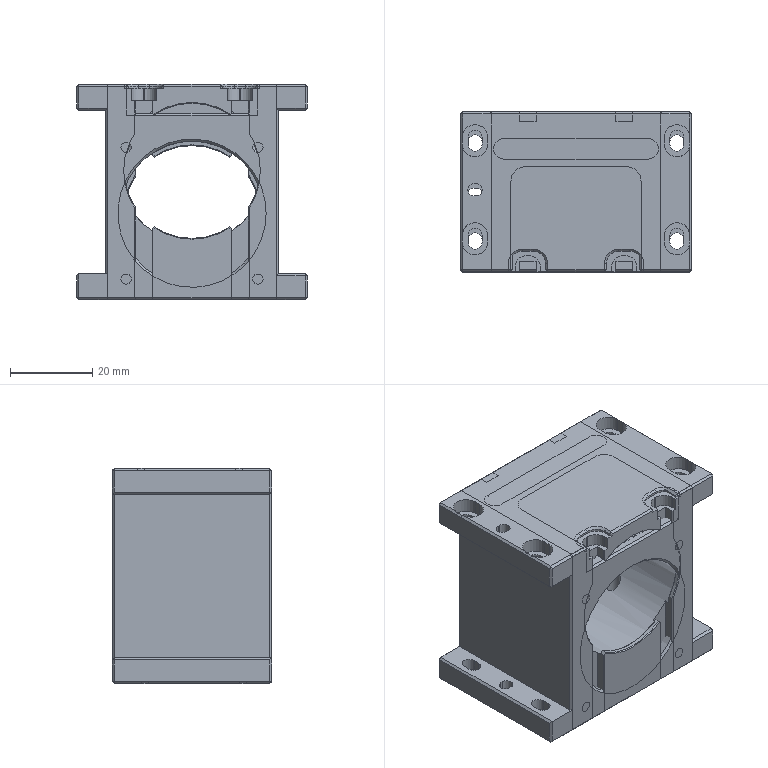NC program | NX | posted with a generic post | part box 56 x 38.8 x 52.3 mm
Lines 2544 to 3538 of 18366:
(轮廓清角-D12 , TOOL : 粗刀D3)
N5056 T16 M6
N5058 G54
N5060 G17 G0 G90 X12.601 Y-4.005 S12000 M3
N5062 G43 Z30.1 H16
N5064 Z-0.7
N5066 G41 G94 G1 X12.8 Y-3.985 F1500. D16
N5068 G3 X13.7 Y-2.99 R1.
N5070 G1 Y2.6
N5072 G3 X12.3 Y4. R1.4
N5074 G1 X6.71
N5076 G3 X5.715 Y3.1 R1.
N5078 G40
N5080 G1 X5.695 Y2.901
N5082 G0 X12.601 Y-4.005 Z-1.4
N5084 G41 G1 X12.8 Y-3.985
N5086 G3 X13.7 Y-2.99 R1.
N5088 G1 Y2.6
N5090 G3 X12.3 Y4. R1.4
N5092 G1 X6.71
N5094 G3 X5.715 Y3.1 R1.
N5096 G40
N5098 G1 X5.695 Y2.901
N5100 G0 X12.601 Y-4.005 Z-2.1
N5102 G41 G1 X12.8 Y-3.985
N5104 G3 X13.7 Y-2.99 R1.
N5106 G1 Y2.6
N5108 G3 X12.3 Y4. R1.4
N5110 G1 X6.71
N5112 G3 X5.715 Y3.1 R1.
N5114 G40
N5116 G1 X5.695 Y2.901
N5118 G0 X12.601 Y-4.005 Z-2.8
N5120 G41 G1 X12.8 Y-3.985
N5122 G3 X13.7 Y-2.99 R1.
N5124 G1 Y2.6
N5126 G3 X12.3 Y4. R1.4
N5128 G1 X6.71
N5130 G3 X5.715 Y3.1 R1.
N5132 G40
N5134 G1 X5.695 Y2.901
N5136 G0 X12.601 Y-4.005 Z-3.5
N5138 G41 G1 X12.8 Y-3.985
N5140 G3 X13.7 Y-2.99 R1.
N5142 G1 Y2.6
N5144 G3 X12.3 Y4. R1.4
N5146 G1 X6.71
N5148 G3 X5.715 Y3.1 R1.
N5150 G40
N5152 G1 X5.695 Y2.901
N5154 G0 X12.601 Y-4.005 Z-4.2
N5156 G41 G1 X12.8 Y-3.985
N5158 G3 X13.7 Y-2.99 R1.
N5160 G1 Y2.6
N5162 G3 X12.3 Y4. R1.4
N5164 G1 X6.71
N5166 G3 X5.715 Y3.1 R1.
N5168 G40
N5170 G1 X5.695 Y2.901
N5172 G0 X12.601 Y-4.005 Z-4.9
N5174 G41 G1 X12.8 Y-3.985
N5176 G3 X13.7 Y-2.99 R1.
N5178 G1 Y2.6
N5180 G3 X12.3 Y4. R1.4
N5182 G1 X6.71
N5184 G3 X5.715 Y3.1 R1.
N5186 G40
N5188 G1 X5.695 Y2.901
N5190 G0 X12.601 Y-4.005 Z-5.6
N5192 G41 G1 X12.8 Y-3.985
N5194 G3 X13.7 Y-2.99 R1.
N5196 G1 Y2.6
N5198 G3 X12.3 Y4. R1.4
N5200 G1 X6.71
N5202 G3 X5.715 Y3.1 R1.
N5204 G40
N5206 G1 X5.695 Y2.901
N5208 G0 X12.601 Y-4.005 Z-6.3
N5210 G41 G1 X12.8 Y-3.985
N5212 G3 X13.7 Y-2.99 R1.
N5214 G1 Y2.6
N5216 G3 X12.3 Y4. R1.4
N5218 G1 X6.71
N5220 G3 X5.715 Y3.1 R1.
N5222 G40
N5224 G1 X5.695 Y2.901
N5226 G0 X12.601 Y-4.005 Z-6.95
N5228 G41 G1 X12.8 Y-3.985
N5230 G3 X13.7 Y-2.99 R1.
N5232 G1 Y2.6
N5234 G3 X12.3 Y4. R1.4
N5236 G1 X6.71
N5238 G3 X5.715 Y3.1 R1.
N5240 G40
N5242 G1 X5.695 Y2.901
N5244 G0 Z30.1
N5246 X-5.695
N5248 Z-0.7
N5250 G41 G1 X-5.715 Y3.1
N5252 G3 X-6.71 Y4. R1.
N5254 G1 X-12.3
N5256 G3 X-13.7 Y2.6 R1.4
N5258 G1 Y-2.99
N5260 G3 X-12.8 Y-3.985 R1.
N5262 G40
N5264 G1 X-12.601 Y-4.005
N5266 G0 X-5.695 Y2.901 Z-1.4
N5268 G41 G1 X-5.715 Y3.1
N5270 G3 X-6.71 Y4. R1.
N5272 G1 X-12.3
N5274 G3 X-13.7 Y2.6 R1.4
N5276 G1 Y-2.99
N5278 G3 X-12.8 Y-3.985 R1.
N5280 G40
N5282 G1 X-12.601 Y-4.005
N5284 G0 X-5.695 Y2.901 Z-2.1
N5286 G41 G1 X-5.715 Y3.1
N5288 G3 X-6.71 Y4. R1.
N5290 G1 X-12.3
N5292 G3 X-13.7 Y2.6 R1.4
N5294 G1 Y-2.99
N5296 G3 X-12.8 Y-3.985 R1.
N5298 G40
N5300 G1 X-12.601 Y-4.005
N5302 G0 X-5.695 Y2.901 Z-2.8
N5304 G41 G1 X-5.715 Y3.1
N5306 G3 X-6.71 Y4. R1.
N5308 G1 X-12.3
N5310 G3 X-13.7 Y2.6 R1.4
N5312 G1 Y-2.99
N5314 G3 X-12.8 Y-3.985 R1.
N5316 G40
N5318 G1 X-12.601 Y-4.005
N5320 G0 X-5.695 Y2.901 Z-3.5
N5322 G41 G1 X-5.715 Y3.1
N5324 G3 X-6.71 Y4. R1.
N5326 G1 X-12.3
N5328 G3 X-13.7 Y2.6 R1.4
N5330 G1 Y-2.99
N5332 G3 X-12.8 Y-3.985 R1.
N5334 G40
N5336 G1 X-12.601 Y-4.005
N5338 G0 X-5.695 Y2.901 Z-4.2
N5340 G41 G1 X-5.715 Y3.1
N5342 G3 X-6.71 Y4. R1.
N5344 G1 X-12.3
N5346 G3 X-13.7 Y2.6 R1.4
N5348 G1 Y-2.99
N5350 G3 X-12.8 Y-3.985 R1.
N5352 G40
N5354 G1 X-12.601 Y-4.005
N5356 G0 X-5.695 Y2.901 Z-4.9
N5358 G41 G1 X-5.715 Y3.1
N5360 G3 X-6.71 Y4. R1.
N5362 G1 X-12.3
N5364 G3 X-13.7 Y2.6 R1.4
N5366 G1 Y-2.99
N5368 G3 X-12.8 Y-3.985 R1.
N5370 G40
N5372 G1 X-12.601 Y-4.005
N5374 G0 X-5.695 Y2.901 Z-5.6
N5376 G41 G1 X-5.715 Y3.1
N5378 G3 X-6.71 Y4. R1.
N5380 G1 X-12.3
N5382 G3 X-13.7 Y2.6 R1.4
N5384 G1 Y-2.99
N5386 G3 X-12.8 Y-3.985 R1.
N5388 G40
N5390 G1 X-12.601 Y-4.005
N5392 G0 X-5.695 Y2.901 Z-6.3
N5394 G41 G1 X-5.715 Y3.1
N5396 G3 X-6.71 Y4. R1.
N5398 G1 X-12.3
N5400 G3 X-13.7 Y2.6 R1.4
N5402 G1 Y-2.99
N5404 G3 X-12.8 Y-3.985 R1.
N5406 G40
N5408 G1 X-12.601 Y-4.005
N5410 G0 X-5.695 Y2.901 Z-6.95
N5412 G41 G1 X-5.715 Y3.1
N5414 G3 X-6.71 Y4. R1.
N5416 G1 X-12.3
N5418 G3 X-13.7 Y2.6 R1.4
N5420 G1 Y-2.99
N5422 G3 X-12.8 Y-3.985 R1.
N5424 G40
N5426 G1 X-12.601 Y-4.005
N5428 G0 Z30.1
(平面铣螺旋开粗 , TOOL : 粗刀D3)
N5430 Z30.5 S10000
N5432 X24.8 Y11.4
N5434 G1 Z3.8 F5000.
N5436 Z0.8 F1300.
N5438 G41 X25.
N5440 G3 X26. Y12.4 R1.
N5442 G1 Y13.2 Z0.787 F1400.
N5444 G3 X24.5 Y14.7 Z0.751 R1.5
N5446 X23. Y13.2 Z0.714 R1.5
N5448 G1 Y11.6 Z0.689
N5450 G3 X24.5 Y10.1 Z0.652 R1.5
N5452 X26. Y11.6 Z0.615 R1.5
N5454 G1 Y13.2 Z0.59
N5456 G3 X24.5 Y14.7 Z0.553 R1.5
N5458 X23. Y13.2 Z0.516 R1.5
N5460 G1 Y11.6 Z0.491
N5462 G3 X24.5 Y10.1 Z0.454 R1.5
N5464 X26. Y11.6 Z0.417 R1.5
N5466 G1 Y13.2 Z0.392
N5468 G3 X24.5 Y14.7 Z0.355 R1.5
N5470 X23. Y13.2 Z0.318 R1.5
N5472 G1 Y11.6 Z0.293
N5474 G3 X24.5 Y10.1 Z0.257 R1.5
N5476 X26. Y11.6 Z0.22 R1.5
N5478 G1 Y13.2 Z0.195
N5480 G3 X24.5 Y14.7 Z0.158 R1.5
N5482 X23. Y13.2 Z0.121 R1.5
N5484 G1 Y11.6 Z0.096
N5486 G3 X24.5 Y10.1 Z0.059 R1.5
N5488 X26. Y11.6 Z0.022 R1.5
N5490 G1 Y13.2 Z-0.003
N5492 G3 X24.5 Y14.7 Z-0.04 R1.5
N5494 X23. Y13.2 Z-0.077 R1.5
N5496 G1 Y11.6 Z-0.102
N5498 G3 X24.5 Y10.1 Z-0.139 R1.5
N5500 X26. Y11.6 Z-0.176 R1.5
N5502 G1 Y13.2 Z-0.201
N5504 G3 X24.5 Y14.7 Z-0.238 R1.5
N5506 X23. Y13.2 Z-0.274 R1.5
N5508 G1 Y11.6 Z-0.299
N5510 G3 X24.5 Y10.1 Z-0.336 R1.5
N5512 X26. Y11.6 Z-0.373 R1.5
N5514 G1 Y13.2 Z-0.398
N5516 G3 X24.5 Y14.7 Z-0.435 R1.5
N5518 X23. Y13.2 Z-0.472 R1.5
N5520 G1 Y11.6 Z-0.497
N5522 G3 X24.5 Y10.1 Z-0.534 R1.5
N5524 X26. Y11.6 Z-0.571 R1.5
N5526 G1 Y13.2 Z-0.596
N5528 G3 X24.5 Y14.7 Z-0.633 R1.5
N5530 X23. Y13.2 Z-0.67 R1.5
N5532 G1 Y11.6 Z-0.695
N5534 G3 X24.5 Y10.1 Z-0.732 R1.5
N5536 X26. Y11.6 Z-0.768 R1.5
N5538 G1 Y13.2 Z-0.793
N5540 G3 X24.5 Y14.7 Z-0.83 R1.5
N5542 X23. Y13.2 Z-0.867 R1.5
N5544 G1 Y11.6 Z-0.892
N5546 G3 X24.5 Y10.1 Z-0.929 R1.5
N5548 X26. Y11.6 Z-0.966 R1.5
N5550 G1 Y13.2 Z-0.991
N5552 G3 X24.5 Y14.7 Z-1.028 R1.5
N5554 X23. Y13.2 Z-1.065 R1.5
N5556 G1 Y11.6 Z-1.09
N5558 G3 X24.5 Y10.1 Z-1.127 R1.5
N5560 X26. Y11.6 Z-1.164 R1.5
N5562 G1 Y13.2 Z-1.189
N5564 G3 X24.5 Y14.7 Z-1.226 R1.5
N5566 X23. Y13.2 Z-1.262 R1.5
N5568 G1 Y11.6 Z-1.288
N5570 G3 X24.5 Y10.1 Z-1.324 R1.5
N5572 X26. Y11.6 Z-1.361 R1.5
N5574 G1 Y13.2 Z-1.386
N5576 G3 X24.5 Y14.7 Z-1.423 R1.5
N5578 X23. Y13.2 Z-1.46 R1.5
N5580 G1 Y11.6 Z-1.485
N5582 G3 X24.5 Y10.1 Z-1.522 R1.5
N5584 X26. Y11.6 Z-1.559 R1.5
N5586 G1 Y13.2 Z-1.584
N5588 G3 X24.5 Y14.7 Z-1.621 R1.5
N5590 X23. Y13.2 Z-1.658 R1.5
N5592 G1 Y11.6 Z-1.683
N5594 G3 X24.5 Y10.1 Z-1.72 R1.5
N5596 X26. Y11.6 Z-1.757 R1.5
N5598 G1 Y13.2 Z-1.782
N5600 G3 X24.5 Y14.7 Z-1.818 R1.5
N5602 X23. Y13.2 Z-1.855 R1.5
N5604 G1 Y11.6 Z-1.88
N5606 G3 X24.5 Y10.1 Z-1.917 R1.5
N5608 X26. Y11.6 Z-1.954 R1.5
N5610 G1 Y13.2 Z-1.979
N5612 G3 X24.5 Y14.7 Z-2.016 R1.5
N5614 X23. Y13.2 Z-2.053 R1.5
N5616 G1 Y11.6 Z-2.078
N5618 G3 X24.5 Y10.1 Z-2.115 R1.5
N5620 X26. Y11.6 Z-2.152 R1.5
N5622 G1 Y13.2 Z-2.177
N5624 G3 X24.5 Y14.7 Z-2.214 R1.5
N5626 X23. Y13.2 Z-2.251 R1.5
N5628 G1 Y11.6 Z-2.276
N5630 G3 X24.5 Y10.1 Z-2.313 R1.5
N5632 X26. Y11.6 Z-2.349 R1.5
N5634 G1 Y13.2 Z-2.374
N5636 G3 X24.5 Y14.7 Z-2.411 R1.5
N5638 X23. Y13.2 Z-2.448 R1.5
N5640 G1 Y11.6 Z-2.473
N5642 G3 X24.5 Y10.1 Z-2.51 R1.5
N5644 X26. Y11.6 Z-2.547 R1.5
N5646 G1 Y13.2 Z-2.572
N5648 G3 X24.5 Y14.7 Z-2.609 R1.5
N5650 X23. Y13.2 Z-2.646 R1.5
N5652 G1 Y11.6 Z-2.671
N5654 G3 X24.5 Y10.1 Z-2.708 R1.5
N5656 X26. Y11.6 Z-2.745 R1.5
N5658 G1 Y13.2 Z-2.77
N5660 G3 X24.5 Y14.7 Z-2.807 R1.5
N5662 X23. Y13.2 Z-2.843 R1.5
N5664 G1 Y11.6 Z-2.868
N5666 G3 X24.5 Y10.1 Z-2.905 R1.5
N5668 X26. Y11.6 Z-2.942 R1.5
N5670 G1 Y13.2 Z-2.967
N5672 G3 X24.5 Y14.7 Z-3.004 R1.5
N5674 X23. Y13.2 Z-3.041 R1.5
N5676 G1 Y11.6 Z-3.066
N5678 G3 X24.5 Y10.1 Z-3.103 R1.5
N5680 X26. Y11.6 Z-3.14 R1.5
N5682 G1 Y13.2 Z-3.165
N5684 G3 X24.5 Y14.7 Z-3.202 R1.5
N5686 X23. Y13.2 Z-3.239 R1.5
N5688 G1 Y11.6 Z-3.264
N5690 G3 X24.5 Y10.1 Z-3.301 R1.5
N5692 X26. Y11.6 Z-3.337 R1.5
N5694 G1 Y12.4 Z-3.35
N5696 Y13.2
N5698 G3 X24.5 Y14.7 R1.5
N5700 X23. Y13.2 R1.5
N5702 G1 Y11.6
N5704 G3 X24.5 Y10.1 R1.5
N5706 X26. Y11.6 R1.5
N5708 G1 Y12.4
N5710 G3 X25. Y13.4 R1.
N5712 G40
N5714 G1 X24.8
N5716 Z-0.35
N5718 G0 Z30.5
N5720 Y-12.4
N5722 G1 Z3.8 F5000.
N5724 Z0.8 F1300.
N5726 G41 X25.
N5728 G3 X26. Y-11.4 R1.
N5730 G1 Y-10.6 Z0.787 F1400.
N5732 G3 X24.5 Y-9.1 Z0.751 R1.5
N5734 X23. Y-10.6 Z0.714 R1.5
N5736 G1 Y-12.2 Z0.689
N5738 G3 X24.5 Y-13.7 Z0.652 R1.5
N5740 X26. Y-12.2 Z0.615 R1.5
N5742 G1 Y-10.6 Z0.59
N5744 G3 X24.5 Y-9.1 Z0.553 R1.5
N5746 X23. Y-10.6 Z0.516 R1.5
N5748 G1 Y-12.2 Z0.491
N5750 G3 X24.5 Y-13.7 Z0.454 R1.5
N5752 X26. Y-12.2 Z0.417 R1.5
N5754 G1 Y-10.6 Z0.392
N5756 G3 X24.5 Y-9.1 Z0.355 R1.5
N5758 X23. Y-10.6 Z0.318 R1.5
N5760 G1 Y-12.2 Z0.293
N5762 G3 X24.5 Y-13.7 Z0.257 R1.5
N5764 X26. Y-12.2 Z0.22 R1.5
N5766 G1 Y-10.6 Z0.195
N5768 G3 X24.5 Y-9.1 Z0.158 R1.5
N5770 X23. Y-10.6 Z0.121 R1.5
N5772 G1 Y-12.2 Z0.096
N5774 G3 X24.5 Y-13.7 Z0.059 R1.5
N5776 X26. Y-12.2 Z0.022 R1.5
N5778 G1 Y-10.6 Z-0.003
N5780 G3 X24.5 Y-9.1 Z-0.04 R1.5
N5782 X23. Y-10.6 Z-0.077 R1.5
N5784 G1 Y-12.2 Z-0.102
N5786 G3 X24.5 Y-13.7 Z-0.139 R1.5
N5788 X26. Y-12.2 Z-0.176 R1.5
N5790 G1 Y-10.6 Z-0.201
N5792 G3 X24.5 Y-9.1 Z-0.238 R1.5
N5794 X23. Y-10.6 Z-0.274 R1.5
N5796 G1 Y-12.2 Z-0.299
N5798 G3 X24.5 Y-13.7 Z-0.336 R1.5
N5800 X26. Y-12.2 Z-0.373 R1.5
N5802 G1 Y-10.6 Z-0.398
N5804 G3 X24.5 Y-9.1 Z-0.435 R1.5
N5806 X23. Y-10.6 Z-0.472 R1.5
N5808 G1 Y-12.2 Z-0.497
N5810 G3 X24.5 Y-13.7 Z-0.534 R1.5
N5812 X26. Y-12.2 Z-0.571 R1.5
N5814 G1 Y-10.6 Z-0.596
N5816 G3 X24.5 Y-9.1 Z-0.633 R1.5
N5818 X23. Y-10.6 Z-0.67 R1.5
N5820 G1 Y-12.2 Z-0.695
N5822 G3 X24.5 Y-13.7 Z-0.732 R1.5
N5824 X26. Y-12.2 Z-0.768 R1.5
N5826 G1 Y-10.6 Z-0.793
N5828 G3 X24.5 Y-9.1 Z-0.83 R1.5
N5830 X23. Y-10.6 Z-0.867 R1.5
N5832 G1 Y-12.2 Z-0.892
N5834 G3 X24.5 Y-13.7 Z-0.929 R1.5
N5836 X26. Y-12.2 Z-0.966 R1.5
N5838 G1 Y-10.6 Z-0.991
N5840 G3 X24.5 Y-9.1 Z-1.028 R1.5
N5842 X23. Y-10.6 Z-1.065 R1.5
N5844 G1 Y-12.2 Z-1.09
N5846 G3 X24.5 Y-13.7 Z-1.127 R1.5
N5848 X26. Y-12.2 Z-1.164 R1.5
N5850 G1 Y-10.6 Z-1.189
N5852 G3 X24.5 Y-9.1 Z-1.226 R1.5
N5854 X23. Y-10.6 Z-1.262 R1.5
N5856 G1 Y-12.2 Z-1.288
N5858 G3 X24.5 Y-13.7 Z-1.324 R1.5
N5860 X26. Y-12.2 Z-1.361 R1.5
N5862 G1 Y-10.6 Z-1.386
N5864 G3 X24.5 Y-9.1 Z-1.423 R1.5
N5866 X23. Y-10.6 Z-1.46 R1.5
N5868 G1 Y-12.2 Z-1.485
N5870 G3 X24.5 Y-13.7 Z-1.522 R1.5
N5872 X26. Y-12.2 Z-1.559 R1.5
N5874 G1 Y-10.6 Z-1.584
N5876 G3 X24.5 Y-9.1 Z-1.621 R1.5
N5878 X23. Y-10.6 Z-1.658 R1.5
N5880 G1 Y-12.2 Z-1.683
N5882 G3 X24.5 Y-13.7 Z-1.72 R1.5
N5884 X26. Y-12.2 Z-1.757 R1.5
N5886 G1 Y-10.6 Z-1.782
N5888 G3 X24.5 Y-9.1 Z-1.818 R1.5
N5890 X23. Y-10.6 Z-1.855 R1.5
N5892 G1 Y-12.2 Z-1.88
N5894 G3 X24.5 Y-13.7 Z-1.917 R1.5
N5896 X26. Y-12.2 Z-1.954 R1.5
N5898 G1 Y-10.6 Z-1.979
N5900 G3 X24.5 Y-9.1 Z-2.016 R1.5
N5902 X23. Y-10.6 Z-2.053 R1.5
N5904 G1 Y-12.2 Z-2.078
N5906 G3 X24.5 Y-13.7 Z-2.115 R1.5
N5908 X26. Y-12.2 Z-2.152 R1.5
N5910 G1 Y-10.6 Z-2.177
N5912 G3 X24.5 Y-9.1 Z-2.214 R1.5
N5914 X23. Y-10.6 Z-2.251 R1.5
N5916 G1 Y-12.2 Z-2.276
N5918 G3 X24.5 Y-13.7 Z-2.313 R1.5
N5920 X26. Y-12.2 Z-2.349 R1.5
N5922 G1 Y-10.6 Z-2.374
N5924 G3 X24.5 Y-9.1 Z-2.411 R1.5
N5926 X23. Y-10.6 Z-2.448 R1.5
N5928 G1 Y-12.2 Z-2.473
N5930 G3 X24.5 Y-13.7 Z-2.51 R1.5
N5932 X26. Y-12.2 Z-2.547 R1.5
N5934 G1 Y-10.6 Z-2.572
N5936 G3 X24.5 Y-9.1 Z-2.609 R1.5
N5938 X23. Y-10.6 Z-2.646 R1.5
N5940 G1 Y-12.2 Z-2.671
N5942 G3 X24.5 Y-13.7 Z-2.708 R1.5
N5944 X26. Y-12.2 Z-2.745 R1.5
N5946 G1 Y-10.6 Z-2.77
N5948 G3 X24.5 Y-9.1 Z-2.807 R1.5
N5950 X23. Y-10.6 Z-2.843 R1.5
N5952 G1 Y-12.2 Z-2.868
N5954 G3 X24.5 Y-13.7 Z-2.905 R1.5
N5956 X26. Y-12.2 Z-2.942 R1.5
N5958 G1 Y-10.6 Z-2.967
N5960 G3 X24.5 Y-9.1 Z-3.004 R1.5
N5962 X23. Y-10.6 Z-3.041 R1.5
N5964 G1 Y-12.2 Z-3.066
N5966 G3 X24.5 Y-13.7 Z-3.103 R1.5
N5968 X26. Y-12.2 Z-3.14 R1.5
N5970 G1 Y-10.6 Z-3.165
N5972 G3 X24.5 Y-9.1 Z-3.202 R1.5
N5974 X23. Y-10.6 Z-3.239 R1.5
N5976 G1 Y-12.2 Z-3.264
N5978 G3 X24.5 Y-13.7 Z-3.301 R1.5
N5980 X26. Y-12.2 Z-3.337 R1.5
N5982 G1 Y-11.4 Z-3.35
N5984 Y-10.6
N5986 G3 X24.5 Y-9.1 R1.5
N5988 X23. Y-10.6 R1.5
N5990 G1 Y-12.2
N5992 G3 X24.5 Y-13.7 R1.5
N5994 X26. Y-12.2 R1.5
N5996 G1 Y-11.4
N5998 G3 X25. Y-10.4 R1.
N6000 G40
N6002 G1 X24.8
N6004 Z-0.35
N6006 G0 Z30.5
N6008 X-24.8
N6010 G1 Z3.8 F5000.
N6012 Z0.8 F1300.
N6014 G41 X-25.
N6016 G3 X-26. Y-11.4 R1.
N6018 G1 Y-12.2 Z0.787 F1400.
N6020 G3 X-24.5 Y-13.7 Z0.751 R1.5
N6022 X-23. Y-12.2 Z0.714 R1.5
N6024 G1 Y-10.6 Z0.689
N6026 G3 X-24.5 Y-9.1 Z0.652 R1.5
N6028 X-26. Y-10.6 Z0.615 R1.5
N6030 G1 Y-12.2 Z0.59
N6032 G3 X-24.5 Y-13.7 Z0.553 R1.5
N6034 X-23. Y-12.2 Z0.516 R1.5
N6036 G1 Y-10.6 Z0.491
N6038 G3 X-24.5 Y-9.1 Z0.454 R1.5
N6040 X-26. Y-10.6 Z0.417 R1.5
N6042 G1 Y-12.2 Z0.392
N6044 G3 X-24.5 Y-13.7 Z0.355 R1.5
N6046 X-23. Y-12.2 Z0.318 R1.5
N6048 G1 Y-10.6 Z0.293
N6050 G3 X-24.5 Y-9.1 Z0.257 R1.5
N6052 X-26. Y-10.6 Z0.22 R1.5
N6054 G1 Y-12.2 Z0.195
N6056 G3 X-24.5 Y-13.7 Z0.158 R1.5
N6058 X-23. Y-12.2 Z0.121 R1.5
N6060 G1 Y-10.6 Z0.096
N6062 G3 X-24.5 Y-9.1 Z0.059 R1.5
N6064 X-26. Y-10.6 Z0.022 R1.5
N6066 G1 Y-12.2 Z-0.003
N6068 G3 X-24.5 Y-13.7 Z-0.04 R1.5
N6070 X-23. Y-12.2 Z-0.077 R1.5
N6072 G1 Y-10.6 Z-0.102
N6074 G3 X-24.5 Y-9.1 Z-0.139 R1.5
N6076 X-26. Y-10.6 Z-0.176 R1.5
N6078 G1 Y-12.2 Z-0.201
N6080 G3 X-24.5 Y-13.7 Z-0.238 R1.5
N6082 X-23. Y-12.2 Z-0.274 R1.5
N6084 G1 Y-10.6 Z-0.299
N6086 G3 X-24.5 Y-9.1 Z-0.336 R1.5
N6088 X-26. Y-10.6 Z-0.373 R1.5
N6090 G1 Y-12.2 Z-0.398
N6092 G3 X-24.5 Y-13.7 Z-0.435 R1.5
N6094 X-23. Y-12.2 Z-0.472 R1.5
N6096 G1 Y-10.6 Z-0.497
N6098 G3 X-24.5 Y-9.1 Z-0.534 R1.5
N6100 X-26. Y-10.6 Z-0.571 R1.5
N6102 G1 Y-12.2 Z-0.596
N6104 G3 X-24.5 Y-13.7 Z-0.633 R1.5
N6106 X-23. Y-12.2 Z-0.67 R1.5
N6108 G1 Y-10.6 Z-0.695
N6110 G3 X-24.5 Y-9.1 Z-0.732 R1.5
N6112 X-26. Y-10.6 Z-0.768 R1.5
N6114 G1 Y-12.2 Z-0.793
N6116 G3 X-24.5 Y-13.7 Z-0.83 R1.5
N6118 X-23. Y-12.2 Z-0.867 R1.5
N6120 G1 Y-10.6 Z-0.892
N6122 G3 X-24.5 Y-9.1 Z-0.929 R1.5
N6124 X-26. Y-10.6 Z-0.966 R1.5
N6126 G1 Y-12.2 Z-0.991
N6128 G3 X-24.5 Y-13.7 Z-1.028 R1.5
N6130 X-23. Y-12.2 Z-1.065 R1.5
N6132 G1 Y-10.6 Z-1.09
N6134 G3 X-24.5 Y-9.1 Z-1.127 R1.5
N6136 X-26. Y-10.6 Z-1.164 R1.5
N6138 G1 Y-12.2 Z-1.189
N6140 G3 X-24.5 Y-13.7 Z-1.226 R1.5
N6142 X-23. Y-12.2 Z-1.262 R1.5
N6144 G1 Y-10.6 Z-1.288
N6146 G3 X-24.5 Y-9.1 Z-1.324 R1.5
N6148 X-26. Y-10.6 Z-1.361 R1.5
N6150 G1 Y-12.2 Z-1.386
N6152 G3 X-24.5 Y-13.7 Z-1.423 R1.5
N6154 X-23. Y-12.2 Z-1.46 R1.5
N6156 G1 Y-10.6 Z-1.485
N6158 G3 X-24.5 Y-9.1 Z-1.522 R1.5
N6160 X-26. Y-10.6 Z-1.559 R1.5
N6162 G1 Y-12.2 Z-1.584
N6164 G3 X-24.5 Y-13.7 Z-1.621 R1.5
N6166 X-23. Y-12.2 Z-1.658 R1.5
N6168 G1 Y-10.6 Z-1.683
N6170 G3 X-24.5 Y-9.1 Z-1.72 R1.5
N6172 X-26. Y-10.6 Z-1.757 R1.5
N6174 G1 Y-12.2 Z-1.782
N6176 G3 X-24.5 Y-13.7 Z-1.818 R1.5
N6178 X-23. Y-12.2 Z-1.855 R1.5
N6180 G1 Y-10.6 Z-1.88
N6182 G3 X-24.5 Y-9.1 Z-1.917 R1.5
N6184 X-26. Y-10.6 Z-1.954 R1.5
N6186 G1 Y-12.2 Z-1.979
N6188 G3 X-24.5 Y-13.7 Z-2.016 R1.5
N6190 X-23. Y-12.2 Z-2.053 R1.5
N6192 G1 Y-10.6 Z-2.078
N6194 G3 X-24.5 Y-9.1 Z-2.115 R1.5
N6196 X-26. Y-10.6 Z-2.152 R1.5
N6198 G1 Y-12.2 Z-2.177
N6200 G3 X-24.5 Y-13.7 Z-2.214 R1.5
N6202 X-23. Y-12.2 Z-2.251 R1.5
N6204 G1 Y-10.6 Z-2.276
N6206 G3 X-24.5 Y-9.1 Z-2.313 R1.5
N6208 X-26. Y-10.6 Z-2.349 R1.5
N6210 G1 Y-12.2 Z-2.374
N6212 G3 X-24.5 Y-13.7 Z-2.411 R1.5
N6214 X-23. Y-12.2 Z-2.448 R1.5
N6216 G1 Y-10.6 Z-2.473
N6218 G3 X-24.5 Y-9.1 Z-2.51 R1.5
N6220 X-26. Y-10.6 Z-2.547 R1.5
N6222 G1 Y-12.2 Z-2.572
N6224 G3 X-24.5 Y-13.7 Z-2.609 R1.5
N6226 X-23. Y-12.2 Z-2.646 R1.5
N6228 G1 Y-10.6 Z-2.671
N6230 G3 X-24.5 Y-9.1 Z-2.708 R1.5
N6232 X-26. Y-10.6 Z-2.745 R1.5
N6234 G1 Y-12.2 Z-2.77
N6236 G3 X-24.5 Y-13.7 Z-2.807 R1.5
N6238 X-23. Y-12.2 Z-2.843 R1.5
N6240 G1 Y-10.6 Z-2.868
N6242 G3 X-24.5 Y-9.1 Z-2.905 R1.5
N6244 X-26. Y-10.6 Z-2.942 R1.5
N6246 G1 Y-12.2 Z-2.967
N6248 G3 X-24.5 Y-13.7 Z-3.004 R1.5
N6250 X-23. Y-12.2 Z-3.041 R1.5
N6252 G1 Y-10.6 Z-3.066
N6254 G3 X-24.5 Y-9.1 Z-3.103 R1.5
N6256 X-26. Y-10.6 Z-3.14 R1.5
N6258 G1 Y-12.2 Z-3.165
N6260 G3 X-24.5 Y-13.7 Z-3.202 R1.5
N6262 X-23. Y-12.2 Z-3.239 R1.5
N6264 G1 Y-10.6 Z-3.264
N6266 G3 X-24.5 Y-9.1 Z-3.301 R1.5
N6268 X-26. Y-10.6 Z-3.337 R1.5
N6270 G1 Y-11.4 Z-3.35
N6272 Y-12.2
N6274 G3 X-24.5 Y-13.7 R1.5
N6276 X-23. Y-12.2 R1.5
N6278 G1 Y-10.6
N6280 G3 X-24.5 Y-9.1 R1.5
N6282 X-26. Y-10.6 R1.5
N6284 G1 Y-11.4
N6286 G3 X-25. Y-12.4 R1.
N6288 G40
N6290 G1 X-24.8
N6292 Z-0.35
N6294 G0 Z30.5
N6296 Y13.4
N6298 G1 Z3.8 F5000.
N6300 Z0.8 F1300.
N6302 G41 X-25.
N6304 G3 X-26. Y12.4 R1.
N6306 G1 Y11.6 Z0.787 F1400.
N6308 G3 X-24.5 Y10.1 Z0.751 R1.5
N6310 X-23. Y11.6 Z0.714 R1.5
N6312 G1 Y13.2 Z0.689
N6314 G3 X-24.5 Y14.7 Z0.652 R1.5
N6316 X-26. Y13.2 Z0.615 R1.5
N6318 G1 Y11.6 Z0.59
N6320 G3 X-24.5 Y10.1 Z0.553 R1.5
N6322 X-23. Y11.6 Z0.516 R1.5
N6324 G1 Y13.2 Z0.491
N6326 G3 X-24.5 Y14.7 Z0.454 R1.5
N6328 X-26. Y13.2 Z0.417 R1.5
N6330 G1 Y11.6 Z0.392
N6332 G3 X-24.5 Y10.1 Z0.355 R1.5
N6334 X-23. Y11.6 Z0.318 R1.5
N6336 G1 Y13.2 Z0.293
N6338 G3 X-24.5 Y14.7 Z0.257 R1.5
N6340 X-26. Y13.2 Z0.22 R1.5
N6342 G1 Y11.6 Z0.195
N6344 G3 X-24.5 Y10.1 Z0.158 R1.5
N6346 X-23. Y11.6 Z0.121 R1.5
N6348 G1 Y13.2 Z0.096
N6350 G3 X-24.5 Y14.7 Z0.059 R1.5
N6352 X-26. Y13.2 Z0.022 R1.5
N6354 G1 Y11.6 Z-0.003
N6356 G3 X-24.5 Y10.1 Z-0.04 R1.5
N6358 X-23. Y11.6 Z-0.077 R1.5
N6360 G1 Y13.2 Z-0.102
N6362 G3 X-24.5 Y14.7 Z-0.139 R1.5
N6364 X-26. Y13.2 Z-0.176 R1.5
N6366 G1 Y11.6 Z-0.201
N6368 G3 X-24.5 Y10.1 Z-0.238 R1.5
N6370 X-23. Y11.6 Z-0.274 R1.5
N6372 G1 Y13.2 Z-0.299
N6374 G3 X-24.5 Y14.7 Z-0.336 R1.5
N6376 X-26. Y13.2 Z-0.373 R1.5
N6378 G1 Y11.6 Z-0.398
N6380 G3 X-24.5 Y10.1 Z-0.435 R1.5
N6382 X-23. Y11.6 Z-0.472 R1.5
N6384 G1 Y13.2 Z-0.497
N6386 G3 X-24.5 Y14.7 Z-0.534 R1.5
N6388 X-26. Y13.2 Z-0.571 R1.5
N6390 G1 Y11.6 Z-0.596
N6392 G3 X-24.5 Y10.1 Z-0.633 R1.5
N6394 X-23. Y11.6 Z-0.67 R1.5
N6396 G1 Y13.2 Z-0.695
N6398 G3 X-24.5 Y14.7 Z-0.732 R1.5
N6400 X-26. Y13.2 Z-0.768 R1.5
N6402 G1 Y11.6 Z-0.793
N6404 G3 X-24.5 Y10.1 Z-0.83 R1.5
N6406 X-23. Y11.6 Z-0.867 R1.5
N6408 G1 Y13.2 Z-0.892
N6410 G3 X-24.5 Y14.7 Z-0.929 R1.5
N6412 X-26. Y13.2 Z-0.966 R1.5
N6414 G1 Y11.6 Z-0.991
N6416 G3 X-24.5 Y10.1 Z-1.028 R1.5
N6418 X-23. Y11.6 Z-1.065 R1.5
N6420 G1 Y13.2 Z-1.09
N6422 G3 X-24.5 Y14.7 Z-1.127 R1.5
N6424 X-26. Y13.2 Z-1.164 R1.5
N6426 G1 Y11.6 Z-1.189
N6428 G3 X-24.5 Y10.1 Z-1.226 R1.5
N6430 X-23. Y11.6 Z-1.262 R1.5
N6432 G1 Y13.2 Z-1.288
N6434 G3 X-24.5 Y14.7 Z-1.324 R1.5
N6436 X-26. Y13.2 Z-1.361 R1.5
N6438 G1 Y11.6 Z-1.386
N6440 G3 X-24.5 Y10.1 Z-1.423 R1.5
N6442 X-23. Y11.6 Z-1.46 R1.5
N6444 G1 Y13.2 Z-1.485
N6446 G3 X-24.5 Y14.7 Z-1.522 R1.5
N6448 X-26. Y13.2 Z-1.559 R1.5
N6450 G1 Y11.6 Z-1.584
N6452 G3 X-24.5 Y10.1 Z-1.621 R1.5
N6454 X-23. Y11.6 Z-1.658 R1.5
N6456 G1 Y13.2 Z-1.683
N6458 G3 X-24.5 Y14.7 Z-1.72 R1.5
N6460 X-26. Y13.2 Z-1.757 R1.5
N6462 G1 Y11.6 Z-1.782
N6464 G3 X-24.5 Y10.1 Z-1.818 R1.5
N6466 X-23. Y11.6 Z-1.855 R1.5
N6468 G1 Y13.2 Z-1.88
N6470 G3 X-24.5 Y14.7 Z-1.917 R1.5
N6472 X-26. Y13.2 Z-1.954 R1.5
N6474 G1 Y11.6 Z-1.979
N6476 G3 X-24.5 Y10.1 Z-2.016 R1.5
N6478 X-23. Y11.6 Z-2.053 R1.5
N6480 G1 Y13.2 Z-2.078
N6482 G3 X-24.5 Y14.7 Z-2.115 R1.5
N6484 X-26. Y13.2 Z-2.152 R1.5
N6486 G1 Y11.6 Z-2.177
N6488 G3 X-24.5 Y10.1 Z-2.214 R1.5
N6490 X-23. Y11.6 Z-2.251 R1.5
N6492 G1 Y13.2 Z-2.276
N6494 G3 X-24.5 Y14.7 Z-2.313 R1.5
N6496 X-26. Y13.2 Z-2.349 R1.5
N6498 G1 Y11.6 Z-2.374
N6500 G3 X-24.5 Y10.1 Z-2.411 R1.5
N6502 X-23. Y11.6 Z-2.448 R1.5
N6504 G1 Y13.2 Z-2.473
N6506 G3 X-24.5 Y14.7 Z-2.51 R1.5
N6508 X-26. Y13.2 Z-2.547 R1.5
N6510 G1 Y11.6 Z-2.572
N6512 G3 X-24.5 Y10.1 Z-2.609 R1.5
N6514 X-23. Y11.6 Z-2.646 R1.5
N6516 G1 Y13.2 Z-2.671
N6518 G3 X-24.5 Y14.7 Z-2.708 R1.5
N6520 X-26. Y13.2 Z-2.745 R1.5
N6522 G1 Y11.6 Z-2.77
N6524 G3 X-24.5 Y10.1 Z-2.807 R1.5
N6526 X-23. Y11.6 Z-2.843 R1.5
N6528 G1 Y13.2 Z-2.868
N6530 G3 X-24.5 Y14.7 Z-2.905 R1.5
N6532 X-26. Y13.2 Z-2.942 R1.5
N6534 G1 Y11.6 Z-2.967
N6536 G3 X-24.5 Y10.1 Z-3.004 R1.5
N6538 X-23. Y11.6 Z-3.041 R1.5
N6540 G1 Y13.2 Z-3.066
N6542 G3 X-24.5 Y14.7 Z-3.103 R1.5
N6544 X-26. Y13.2 Z-3.14 R1.5
N6546 G1 Y11.6 Z-3.165
N6548 G3 X-24.5 Y10.1 Z-3.202 R1.5
N6550 X-23. Y11.6 Z-3.239 R1.5
N6552 G1 Y13.2 Z-3.264
N6554 G3 X-24.5 Y14.7 Z-3.301 R1.5
N6556 X-26. Y13.2 Z-3.337 R1.5
N6558 G1 Y12.4 Z-3.35
N6560 Y11.6
N6562 G3 X-24.5 Y10.1 R1.5
N6564 X-23. Y11.6 R1.5
N6566 G1 Y13.2
N6568 G3 X-24.5 Y14.7 R1.5
N6570 X-26. Y13.2 R1.5
N6572 G1 Y12.4
N6574 G3 X-25. Y11.4 R1.
N6576 G40
N6578 G1 X-24.8
N6580 Z-0.35
N6582 G0 Z30.5
(轮廓开粗 , TOOL : 粗刀D3)
N6584 G18 Y49.55 S8500
N6586 X12.05 Z2.
N6588 Y19.206
N6590 G41 G1 Z0. F2000.
N6592 Z-48.3
N6594 G3 X11.7 Z-48.65 R0.35
N6596 X11.35 Z-48.3 R0.35
N6598 G1 Z0.
N6600 Z1.8
N6602 G40
N6604 Z2.
N6606 G0 X12.05 Y19.012
N6608 G41 G1 Z0.
N6610 Z-48.3
N6612 G3 X11.7 Z-48.65 R0.35
N6614 X11.35 Z-48.3 R0.35
N6616 G1 Z0.
N6618 Z1.8
N6620 G40
N6622 Z2.
N6624 G0 X12.05 Y18.818
N6626 G41 G1 Z0.
N6628 Z-48.3
N6630 G3 X11.7 Z-48.65 R0.35
N6632 X11.35 Z-48.3 R0.35
N6634 G1 Z0.
N6636 Z1.8
N6638 G40
N6640 Z2.
N6642 G0 X12.05 Y18.623
N6644 G41 G1 Z0.
N6646 Z-48.3
N6648 G3 X11.7 Z-48.65 R0.35
N6650 X11.35 Z-48.3 R0.35
N6652 G1 Z0.
N6654 Z1.8
N6656 G40
N6658 Z2.
N6660 G0 X12.05 Y18.429
N6662 G41 G1 Z0.
N6664 Z-48.3
N6666 G3 X11.7 Z-48.65 R0.35
N6668 X11.35 Z-48.3 R0.35
N6670 G1 Z0.
N6672 Z1.8
N6674 G40
N6676 Z2.
N6678 G0 X12.05 Y18.235
N6680 G41 G1 Z0.
N6682 Z-48.3
N6684 G3 X11.7 Z-48.65 R0.35
N6686 X11.35 Z-48.3 R0.35
N6688 G1 Z0.
N6690 Z1.8
N6692 G40
N6694 Z2.
N6696 G0 X12.05 Y18.041
N6698 G41 G1 Z0.
N6700 Z-48.3
N6702 G3 X11.7 Z-48.65 R0.35
N6704 X11.35 Z-48.3 R0.35
N6706 G1 Z0.
N6708 Z1.8
N6710 G40
N6712 Z2.
N6714 G0 X12.05 Y17.847
N6716 G41 G1 Z0.
N6718 Z-48.3
N6720 G3 X11.7 Z-48.65 R0.35
N6722 X11.35 Z-48.3 R0.35
N6724 G1 Z0.
N6726 Z1.8
N6728 G40
N6730 Z2.
N6732 G0 X12.05 Y17.653
N6734 G41 G1 Z0.
N6736 Z-48.3
N6738 G3 X11.7 Z-48.65 R0.35
N6740 X11.35 Z-48.3 R0.35
N6742 G1 Z0.
N6744 Z1.8
N6746 G40
N6748 Z2.
N6750 G0 X12.05 Y17.458
N6752 G41 G1 Z0.
N6754 Z-48.3
N6756 G3 X11.7 Z-48.65 R0.35
N6758 X11.35 Z-48.3 R0.35
N6760 G1 Z0.
N6762 Z1.8
N6764 G40
N6766 Z2.
N6768 G0 X12.05 Y17.264
N6770 G41 G1 Z0.
N6772 Z-48.3
N6774 G3 X11.7 Z-48.65 R0.35
N6776 X11.35 Z-48.3 R0.35
N6778 G1 Z0.
N6780 Z1.8
N6782 G40
N6784 Z2.
N6786 G0 X12.05 Y17.07
N6788 G41 G1 Z0.
N6790 Z-48.3
N6792 G3 X11.7 Z-48.65 R0.35
N6794 X11.35 Z-48.3 R0.35
N6796 G1 Z0.
N6798 Z1.8
N6800 G40
N6802 Z2.
N6804 G0 Y49.55
N6806 X-11.35
N6808 Y19.206
N6810 G41 G1 Z0.
N6812 Z-48.3
N6814 G3 X-11.7 Z-48.65 R0.35
N6816 X-12.05 Z-48.3 R0.35
N6818 G1 Z0.
N6820 Z1.8
N6822 G40
N6824 Z2.
N6826 G0 X-11.35 Y19.012
N6828 G41 G1 Z0.
N6830 Z-48.3
N6832 G3 X-11.7 Z-48.65 R0.35
N6834 X-12.05 Z-48.3 R0.35
N6836 G1 Z0.
N6838 Z1.8
N6840 G40
N6842 Z2.
N6844 G0 X-11.35 Y18.818
N6846 G41 G1 Z0.
N6848 Z-48.3
N6850 G3 X-11.7 Z-48.65 R0.35
N6852 X-12.05 Z-48.3 R0.35
N6854 G1 Z0.
N6856 Z1.8
N6858 G40
N6860 Z2.
N6862 G0 X-11.35 Y18.623
N6864 G41 G1 Z0.
N6866 Z-48.3
N6868 G3 X-11.7 Z-48.65 R0.35
N6870 X-12.05 Z-48.3 R0.35
N6872 G1 Z0.
N6874 Z1.8
N6876 G40
N6878 Z2.
N6880 G0 X-11.35 Y18.429
N6882 G41 G1 Z0.
N6884 Z-48.3
N6886 G3 X-11.7 Z-48.65 R0.35
N6888 X-12.05 Z-48.3 R0.35
N6890 G1 Z0.
N6892 Z1.8
N6894 G40
N6896 Z2.
N6898 G0 X-11.35 Y18.235
N6900 G41 G1 Z0.
N6902 Z-48.3
N6904 G3 X-11.7 Z-48.65 R0.35
N6906 X-12.05 Z-48.3 R0.35
N6908 G1 Z0.
N6910 Z1.8
N6912 G40
N6914 Z2.
N6916 G0 X-11.35 Y18.041
N6918 G41 G1 Z0.
N6920 Z-48.3
N6922 G3 X-11.7 Z-48.65 R0.35
N6924 X-12.05 Z-48.3 R0.35
N6926 G1 Z0.
N6928 Z1.8
N6930 G40
N6932 Z2.
N6934 G0 X-11.35 Y17.847
N6936 G41 G1 Z0.
N6938 Z-48.3
N6940 G3 X-11.7 Z-48.65 R0.35
N6942 X-12.05 Z-48.3 R0.35
N6944 G1 Z0.
N6946 Z1.8
N6948 G40
N6950 Z2.
N6952 G0 X-11.35 Y17.653
N6954 G41 G1 Z0.
N6956 Z-48.3
N6958 G3 X-11.7 Z-48.65 R0.35
N6960 X-12.05 Z-48.3 R0.35
N6962 G1 Z0.
N6964 Z1.8
N6966 G40
N6968 Z2.
N6970 G0 X-11.35 Y17.458
N6972 G41 G1 Z0.
N6974 Z-48.3
N6976 G3 X-11.7 Z-48.65 R0.35
N6978 X-12.05 Z-48.3 R0.35
N6980 G1 Z0.
N6982 Z1.8
N6984 G40
N6986 Z2.
N6988 G0 X-11.35 Y17.264
N6990 G41 G1 Z0.
N6992 Z-48.3
N6994 G3 X-11.7 Z-48.65 R0.35
N6996 X-12.05 Z-48.3 R0.35
N6998 G1 Z0.
N7000 Z1.8
N7002 G40
N7004 Z2.
N7006 G0 X-11.35 Y17.07
N7008 G41 G1 Z0.
N7010 Z-48.3
N7012 G3 X-11.7 Z-48.65 R0.35
N7014 X-12.05 Z-48.3 R0.35
N7016 G1 Z0.
N7018 Z1.8
N7020 G40
N7022 Z2.
N7024 G0 Y49.55
N7026 M5